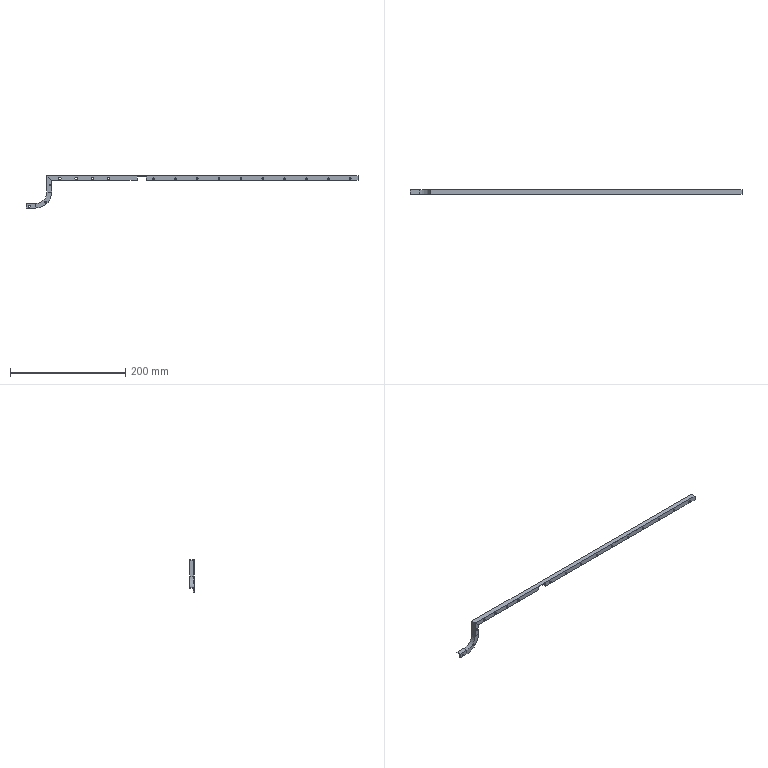Part | STEP file | 1-01.4 symmetric part | 1 solid | 47 faces | box 577.1 x 8 x 56 mm | volume 13016 mm3 | plane 27 | cylinder 20 | commonest cylinder face diameters 3 x13 4 x4 40 x1 43 x1 56 x1